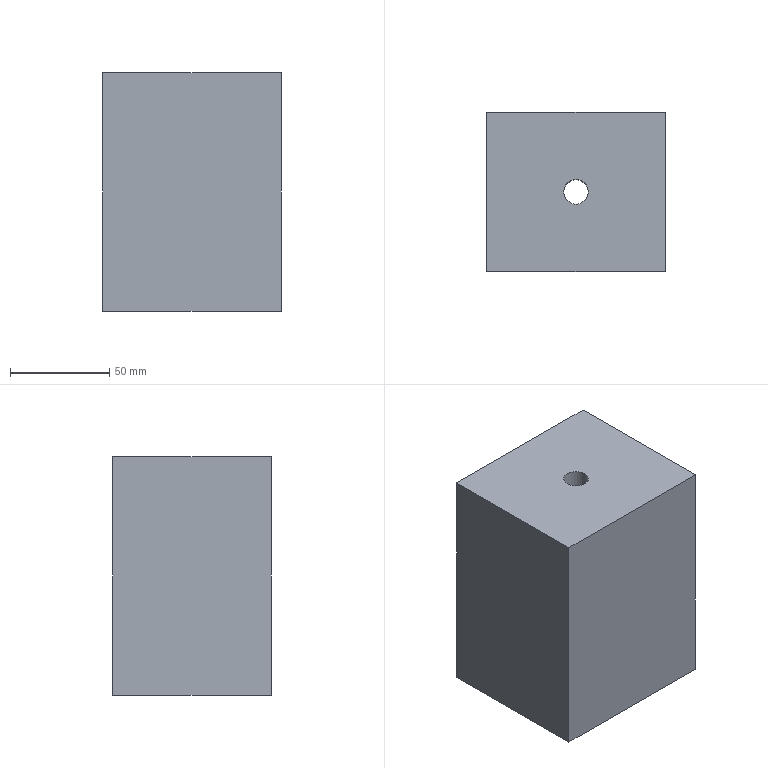Part | SolidWorks | features Extrusion 1, ICE 1 | 1 solid | 8 faces | box 90 x 80 x 120 mm | volume 849508 mm3 | plane 6 | cylinder 2 | commonest cylinder face diameters 12.4 x2
STEP:
#1=CARTESIAN_POINT('',(-6.2,0.,-60.));
#2=VERTEX_POINT('',#1);
#3=CARTESIAN_POINT('',(6.2,0.,-60.));
#4=VERTEX_POINT('',#3);
#5=CARTESIAN_POINT('',(0.,0.,-60.));
#6=DIRECTION('',(0.,0.,1.));
#7=DIRECTION('',(1.,0.,0.));
#8=AXIS2_PLACEMENT_3D('',#5,#6,#7);
#9=CIRCLE('',#8,6.2);
#10=EDGE_CURVE('',#2,#4,#9,.T.);
#11=ORIENTED_EDGE('',*,*,#10,.F.);
#12=CARTESIAN_POINT('',(-6.2,0.,60.));
#13=VERTEX_POINT('',#12);
#14=CARTESIAN_POINT('',(-6.2,0.,-80.));
#15=DIRECTION('',(0.,0.,1.));
#16=VECTOR('',#15,1000.);
#17=LINE('',#14,#16);
#18=EDGE_CURVE('',#2,#13,#17,.T.);
#19=ORIENTED_EDGE('',*,*,#18,.T.);
#20=CARTESIAN_POINT('',(6.2,0.,60.));
#21=VERTEX_POINT('',#20);
#22=CARTESIAN_POINT('',(0.,0.,60.));
#23=DIRECTION('',(0.,0.,1.));
#24=DIRECTION('',(1.,0.,0.));
#25=AXIS2_PLACEMENT_3D('',#22,#23,#24);
#26=CIRCLE('',#25,6.2);
#27=EDGE_CURVE('',#13,#21,#26,.T.);
#28=ORIENTED_EDGE('',*,*,#27,.T.);
#29=CARTESIAN_POINT('',(6.2,0.,-80.));
#30=DIRECTION('',(0.,0.,1.));
#31=VECTOR('',#30,1000.);
#32=LINE('',#29,#31);
#33=EDGE_CURVE('',#4,#21,#32,.T.);
#34=ORIENTED_EDGE('',*,*,#33,.F.);
#35=EDGE_LOOP('',(#11,#19,#28,#34));
#36=FACE_OUTER_BOUND('',#35,.T.);
#37=CARTESIAN_POINT('',(0.,0.,-80.));
#38=DIRECTION('',(0.,0.,1.));
#39=DIRECTION('',(1.,0.,0.));
#40=AXIS2_PLACEMENT_3D('',#37,#38,#39);
#41=CYLINDRICAL_SURFACE('',#40,6.2);
#42=ADVANCED_FACE('',(#36),#41,.F.);
#43=CARTESIAN_POINT('',(-45.,40.,60.));
#44=VERTEX_POINT('',#43);
#45=CARTESIAN_POINT('',(-45.,-40.,60.));
#46=VERTEX_POINT('',#45);
#47=CARTESIAN_POINT('',(-45.,40.,60.));
#48=DIRECTION('',(0.,-1.,0.));
#49=VECTOR('',#48,1000.);
#50=LINE('',#47,#49);
#51=EDGE_CURVE('',#44,#46,#50,.T.);
#52=ORIENTED_EDGE('',*,*,#51,.F.);
#53=CARTESIAN_POINT('',(-45.,40.,-60.));
#54=VERTEX_POINT('',#53);
#55=CARTESIAN_POINT('',(-45.,40.,-60.));
#56=DIRECTION('',(0.,0.,1.));
#57=VECTOR('',#56,1000.);
#58=LINE('',#55,#57);
#59=EDGE_CURVE('',#54,#44,#58,.T.);
#60=ORIENTED_EDGE('',*,*,#59,.F.);
#61=CARTESIAN_POINT('',(-45.,-40.,-60.));
#62=VERTEX_POINT('',#61);
#63=CARTESIAN_POINT('',(-45.,40.,-60.));
#64=DIRECTION('',(0.,-1.,0.));
#65=VECTOR('',#64,1000.);
#66=LINE('',#63,#65);
#67=EDGE_CURVE('',#54,#62,#66,.T.);
#68=ORIENTED_EDGE('',*,*,#67,.T.);
#69=CARTESIAN_POINT('',(-45.,-40.,-60.));
#70=DIRECTION('',(0.,0.,1.));
#71=VECTOR('',#70,1000.);
#72=LINE('',#69,#71);
#73=EDGE_CURVE('',#62,#46,#72,.T.);
#74=ORIENTED_EDGE('',*,*,#73,.T.);
#75=EDGE_LOOP('',(#52,#60,#68,#74));
#76=FACE_OUTER_BOUND('',#75,.T.);
#77=CARTESIAN_POINT('',(-45.,40.,-60.));
#78=DIRECTION('',(-1.,0.,0.));
#79=DIRECTION('',(0.,0.,1.));
#80=AXIS2_PLACEMENT_3D('',#77,#78,#79);
#81=PLANE('',#80);
#82=ADVANCED_FACE('',(#76),#81,.T.);
#83=CARTESIAN_POINT('',(45.,40.,60.));
#84=VERTEX_POINT('',#83);
#85=CARTESIAN_POINT('',(45.,40.,60.));
#86=DIRECTION('',(-1.,0.,0.));
#87=VECTOR('',#86,1000.);
#88=LINE('',#85,#87);
#89=EDGE_CURVE('',#84,#44,#88,.T.);
#90=ORIENTED_EDGE('',*,*,#89,.F.);
#91=CARTESIAN_POINT('',(45.,40.,-60.));
#92=VERTEX_POINT('',#91);
#93=CARTESIAN_POINT('',(45.,40.,-60.));
#94=DIRECTION('',(0.,0.,1.));
#95=VECTOR('',#94,1000.);
#96=LINE('',#93,#95);
#97=EDGE_CURVE('',#92,#84,#96,.T.);
#98=ORIENTED_EDGE('',*,*,#97,.F.);
#99=CARTESIAN_POINT('',(45.,40.,-60.));
#100=DIRECTION('',(-1.,0.,0.));
#101=VECTOR('',#100,1000.);
#102=LINE('',#99,#101);
#103=EDGE_CURVE('',#92,#54,#102,.T.);
#104=ORIENTED_EDGE('',*,*,#103,.T.);
#105=ORIENTED_EDGE('',*,*,#59,.T.);
#106=EDGE_LOOP('',(#90,#98,#104,#105));
#107=FACE_OUTER_BOUND('',#106,.T.);
#108=CARTESIAN_POINT('',(45.,40.,-60.));
#109=DIRECTION('',(0.,1.,0.));
#110=DIRECTION('',(0.,0.,1.));
#111=AXIS2_PLACEMENT_3D('',#108,#109,#110);
#112=PLANE('',#111);
#113=ADVANCED_FACE('',(#107),#112,.T.);
#114=CARTESIAN_POINT('',(45.,-40.,60.));
#115=VERTEX_POINT('',#114);
#116=CARTESIAN_POINT('',(45.,-40.,60.));
#117=DIRECTION('',(0.,1.,0.));
#118=VECTOR('',#117,1000.);
#119=LINE('',#116,#118);
#120=EDGE_CURVE('',#115,#84,#119,.T.);
#121=ORIENTED_EDGE('',*,*,#120,.F.);
#122=CARTESIAN_POINT('',(45.,-40.,-60.));
#123=VERTEX_POINT('',#122);
#124=CARTESIAN_POINT('',(45.,-40.,-60.));
#125=DIRECTION('',(0.,0.,1.));
#126=VECTOR('',#125,1000.);
#127=LINE('',#124,#126);
#128=EDGE_CURVE('',#123,#115,#127,.T.);
#129=ORIENTED_EDGE('',*,*,#128,.F.);
#130=CARTESIAN_POINT('',(45.,-40.,-60.));
#131=DIRECTION('',(0.,1.,0.));
#132=VECTOR('',#131,1000.);
#133=LINE('',#130,#132);
#134=EDGE_CURVE('',#123,#92,#133,.T.);
#135=ORIENTED_EDGE('',*,*,#134,.T.);
#136=ORIENTED_EDGE('',*,*,#97,.T.);
#137=EDGE_LOOP('',(#121,#129,#135,#136));
#138=FACE_OUTER_BOUND('',#137,.T.);
#139=CARTESIAN_POINT('',(45.,-40.,-60.));
#140=DIRECTION('',(1.,0.,0.));
#141=DIRECTION('',(0.,0.,-1.));
#142=AXIS2_PLACEMENT_3D('',#139,#140,#141);
#143=PLANE('',#142);
#144=ADVANCED_FACE('',(#138),#143,.T.);
#145=CARTESIAN_POINT('',(-45.,-40.,60.));
#146=DIRECTION('',(1.,0.,0.));
#147=VECTOR('',#146,1000.);
#148=LINE('',#145,#147);
#149=EDGE_CURVE('',#46,#115,#148,.T.);
#150=ORIENTED_EDGE('',*,*,#149,.F.);
#151=ORIENTED_EDGE('',*,*,#73,.F.);
#152=CARTESIAN_POINT('',(-45.,-40.,-60.));
#153=DIRECTION('',(1.,0.,0.));
#154=VECTOR('',#153,1000.);
#155=LINE('',#152,#154);
#156=EDGE_CURVE('',#62,#123,#155,.T.);
#157=ORIENTED_EDGE('',*,*,#156,.T.);
#158=ORIENTED_EDGE('',*,*,#128,.T.);
#159=EDGE_LOOP('',(#150,#151,#157,#158));
#160=FACE_OUTER_BOUND('',#159,.T.);
#161=CARTESIAN_POINT('',(-45.,-40.,-60.));
#162=DIRECTION('',(0.,-1.,0.));
#163=DIRECTION('',(0.,0.,-1.));
#164=AXIS2_PLACEMENT_3D('',#161,#162,#163);
#165=PLANE('',#164);
#166=ADVANCED_FACE('',(#160),#165,.T.);
#167=CARTESIAN_POINT('',(0.,0.,-60.));
#168=DIRECTION('',(0.,0.,1.));
#169=DIRECTION('',(1.,0.,0.));
#170=AXIS2_PLACEMENT_3D('',#167,#168,#169);
#171=CIRCLE('',#170,6.2);
#172=EDGE_CURVE('',#4,#2,#171,.T.);
#173=ORIENTED_EDGE('',*,*,#172,.T.);
#174=ORIENTED_EDGE('',*,*,#10,.T.);
#175=EDGE_LOOP('',(#173,#174));
#176=FACE_BOUND('',#175,.T.);
#177=ORIENTED_EDGE('',*,*,#67,.F.);
#178=ORIENTED_EDGE('',*,*,#103,.F.);
#179=ORIENTED_EDGE('',*,*,#134,.F.);
#180=ORIENTED_EDGE('',*,*,#156,.F.);
#181=EDGE_LOOP('',(#177,#178,#179,#180));
#182=FACE_OUTER_BOUND('',#181,.T.);
#183=CARTESIAN_POINT('',(0.,0.,-60.));
#184=DIRECTION('',(0.,0.,1.));
#185=DIRECTION('',(1.,0.,0.));
#186=AXIS2_PLACEMENT_3D('',#183,#184,#185);
#187=PLANE('',#186);
#188=ADVANCED_FACE('',(#176,#182),#187,.F.);
#189=CARTESIAN_POINT('',(0.,0.,60.));
#190=DIRECTION('',(0.,0.,1.));
#191=DIRECTION('',(1.,0.,0.));
#192=AXIS2_PLACEMENT_3D('',#189,#190,#191);
#193=CIRCLE('',#192,6.2);
#194=EDGE_CURVE('',#21,#13,#193,.T.);
#195=ORIENTED_EDGE('',*,*,#194,.F.);
#196=ORIENTED_EDGE('',*,*,#27,.F.);
#197=EDGE_LOOP('',(#195,#196));
#198=FACE_BOUND('',#197,.T.);
#199=ORIENTED_EDGE('',*,*,#51,.T.);
#200=ORIENTED_EDGE('',*,*,#149,.T.);
#201=ORIENTED_EDGE('',*,*,#120,.T.);
#202=ORIENTED_EDGE('',*,*,#89,.T.);
#203=EDGE_LOOP('',(#199,#200,#201,#202));
#204=FACE_OUTER_BOUND('',#203,.T.);
#205=CARTESIAN_POINT('',(0.,0.,60.));
#206=DIRECTION('',(0.,0.,1.));
#207=DIRECTION('',(1.,0.,0.));
#208=AXIS2_PLACEMENT_3D('',#205,#206,#207);
#209=PLANE('',#208);
#210=ADVANCED_FACE('',(#198,#204),#209,.T.);
#211=ORIENTED_EDGE('',*,*,#18,.F.);
#212=ORIENTED_EDGE('',*,*,#172,.F.);
#213=ORIENTED_EDGE('',*,*,#33,.T.);
#214=ORIENTED_EDGE('',*,*,#194,.T.);
#215=EDGE_LOOP('',(#211,#212,#213,#214));
#216=FACE_OUTER_BOUND('',#215,.T.);
#217=CARTESIAN_POINT('',(0.,0.,-80.));
#218=DIRECTION('',(0.,0.,1.));
#219=DIRECTION('',(1.,0.,0.));
#220=AXIS2_PLACEMENT_3D('',#217,#218,#219);
#221=CYLINDRICAL_SURFACE('',#220,6.2);
#222=ADVANCED_FACE('',(#216),#221,.F.);
#223=CLOSED_SHELL('',(#42,#82,#113,#144,#166,#188,#210,#222));
#224=MANIFOLD_SOLID_BREP('',#223);
#225=CARTESIAN_POINT('',(0.,0.,0.));
#226=DIRECTION('',(0.,0.,1.));
#227=DIRECTION('',(1.,0.,0.));
#228=AXIS2_PLACEMENT_3D('',#225,#226,#227);
#229=(LENGTH_UNIT()NAMED_UNIT(*)SI_UNIT(.MILLI.,.METRE.));
#230=UNCERTAINTY_MEASURE_WITH_UNIT(LENGTH_MEASURE(0.00001),#229,'','');
#231=(NAMED_UNIT(*)PLANE_ANGLE_UNIT()SI_UNIT($,.RADIAN.));
#232=(NAMED_UNIT(*)SI_UNIT($,.STERADIAN.)SOLID_ANGLE_UNIT());
#233=(GEOMETRIC_REPRESENTATION_CONTEXT(3)GLOBAL_UNCERTAINTY_ASSIGNED_CONTEXT((#230))GLOBAL_UNIT_ASSIGNED_CONTEXT((#229,#231,#232))REPRESENTATION_CONTEXT('',''));
#234=ADVANCED_BREP_SHAPE_REPRESENTATION('',(#224,#228),#233);